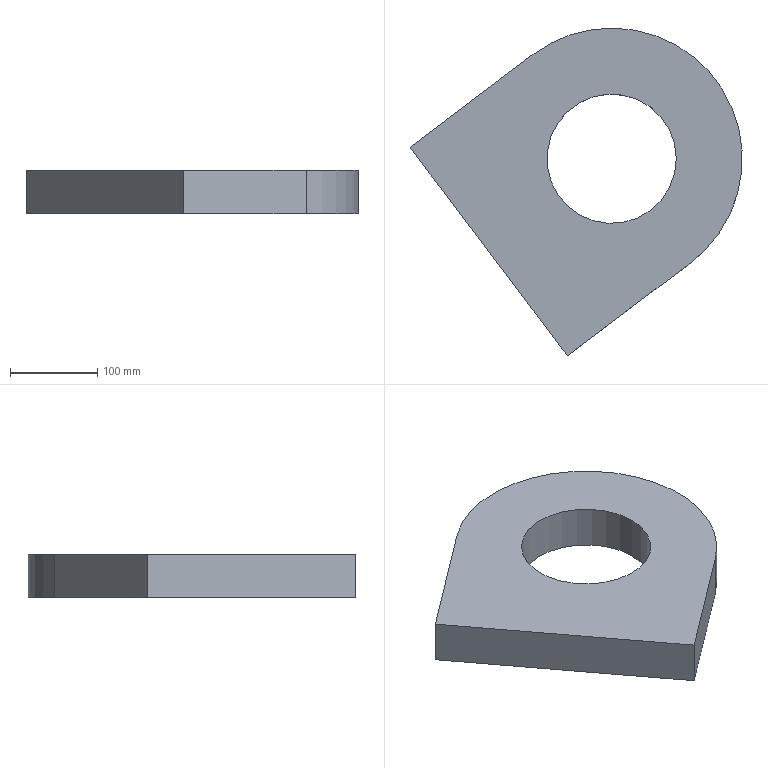Part | NX | features 底座(默认<按焊接>) 2 | 1 solid | 7 faces | box 381.454 x 376.184 x 50 mm | volume 3554006 mm3 | plane 5 | cylinder 2 | commonest cylinder face diameters 148.4 x1 300 x1
STEP:
#1=CARTESIAN_POINT('',(2456.913,471.615,-412.));
#2=VERTEX_POINT('',#1);
#3=CARTESIAN_POINT('',(2637.457,232.025,-412.));
#4=VERTEX_POINT('',#3);
#5=CARTESIAN_POINT('',(2547.185,351.82,-412.));
#6=DIRECTION('',(0.,0.,-1.));
#7=DIRECTION('',(-1.,0.,0.));
#8=AXIS2_PLACEMENT_3D('',#5,#6,#7);
#9=CIRCLE('',#8,150.);
#10=EDGE_CURVE('',#2,#4,#9,.T.);
#11=ORIENTED_EDGE('',*,*,#10,.T.);
#12=CARTESIAN_POINT('',(2637.457,232.025,-462.));
#13=VERTEX_POINT('',#12);
#14=CARTESIAN_POINT('',(2637.457,232.025,-462.));
#15=DIRECTION('',(0.,0.,1.));
#16=VECTOR('',#15,1000.);
#17=LINE('',#14,#16);
#18=EDGE_CURVE('',#13,#4,#17,.T.);
#19=ORIENTED_EDGE('',*,*,#18,.F.);
#20=CARTESIAN_POINT('',(2456.913,471.615,-462.));
#21=VERTEX_POINT('',#20);
#22=CARTESIAN_POINT('',(2547.185,351.82,-462.));
#23=DIRECTION('',(0.,0.,-1.));
#24=DIRECTION('',(-1.,0.,0.));
#25=AXIS2_PLACEMENT_3D('',#22,#23,#24);
#26=CIRCLE('',#25,150.);
#27=EDGE_CURVE('',#21,#13,#26,.T.);
#28=ORIENTED_EDGE('',*,*,#27,.F.);
#29=CARTESIAN_POINT('',(2456.913,471.615,-462.));
#30=DIRECTION('',(0.,0.,1.));
#31=VECTOR('',#30,1000.);
#32=LINE('',#29,#31);
#33=EDGE_CURVE('',#21,#2,#32,.T.);
#34=ORIENTED_EDGE('',*,*,#33,.T.);
#35=EDGE_LOOP('',(#11,#19,#28,#34));
#36=FACE_BOUND('',#35,.T.);
#37=CARTESIAN_POINT('',(2547.185,351.82,-462.));
#38=DIRECTION('',(0.,0.,1.));
#39=DIRECTION('',(1.,0.,0.));
#40=AXIS2_PLACEMENT_3D('',#37,#38,#39);
#41=CYLINDRICAL_SURFACE('',#40,150.);
#42=ADVANCED_FACE('',(#36),#41,.T.);
#43=CARTESIAN_POINT('',(2496.276,125.636,-412.));
#44=VERTEX_POINT('',#43);
#45=CARTESIAN_POINT('',(2637.457,232.025,-412.));
#46=DIRECTION('',(-0.7986,-0.6018,0.));
#47=VECTOR('',#46,1000.);
#48=LINE('',#45,#47);
#49=EDGE_CURVE('',#4,#44,#48,.T.);
#50=ORIENTED_EDGE('',*,*,#49,.T.);
#51=CARTESIAN_POINT('',(2496.276,125.636,-462.));
#52=VERTEX_POINT('',#51);
#53=CARTESIAN_POINT('',(2496.276,125.636,-462.));
#54=DIRECTION('',(0.,0.,1.));
#55=VECTOR('',#54,1000.);
#56=LINE('',#53,#55);
#57=EDGE_CURVE('',#52,#44,#56,.T.);
#58=ORIENTED_EDGE('',*,*,#57,.F.);
#59=CARTESIAN_POINT('',(2637.457,232.025,-462.));
#60=DIRECTION('',(-0.7986,-0.6018,0.));
#61=VECTOR('',#60,1000.);
#62=LINE('',#59,#61);
#63=EDGE_CURVE('',#13,#52,#62,.T.);
#64=ORIENTED_EDGE('',*,*,#63,.F.);
#65=ORIENTED_EDGE('',*,*,#18,.T.);
#66=EDGE_LOOP('',(#50,#58,#64,#65));
#67=FACE_BOUND('',#66,.T.);
#68=CARTESIAN_POINT('',(2637.457,232.025,-462.));
#69=DIRECTION('',(-0.6018,0.7986,0.));
#70=DIRECTION('',(-0.7986,-0.6018,0.));
#71=AXIS2_PLACEMENT_3D('',#68,#69,#70);
#72=PLANE('',#71);
#73=ADVANCED_FACE('',(#67),#72,.F.);
#74=CARTESIAN_POINT('',(2315.731,365.227,-412.));
#75=VERTEX_POINT('',#74);
#76=CARTESIAN_POINT('',(2315.731,365.227,-412.));
#77=DIRECTION('',(-0.6018,0.7986,0.));
#78=VECTOR('',#77,1000.);
#79=LINE('',#76,#78);
#80=EDGE_CURVE('',#44,#75,#79,.T.);
#81=ORIENTED_EDGE('',*,*,#80,.T.);
#82=CARTESIAN_POINT('',(2315.731,365.227,-462.));
#83=VERTEX_POINT('',#82);
#84=CARTESIAN_POINT('',(2315.731,365.227,-462.));
#85=DIRECTION('',(0.,0.,1.));
#86=VECTOR('',#85,1000.);
#87=LINE('',#84,#86);
#88=EDGE_CURVE('',#83,#75,#87,.T.);
#89=ORIENTED_EDGE('',*,*,#88,.F.);
#90=CARTESIAN_POINT('',(2315.731,365.227,-462.));
#91=DIRECTION('',(-0.6018,0.7986,0.));
#92=VECTOR('',#91,1000.);
#93=LINE('',#90,#92);
#94=EDGE_CURVE('',#52,#83,#93,.T.);
#95=ORIENTED_EDGE('',*,*,#94,.F.);
#96=ORIENTED_EDGE('',*,*,#57,.T.);
#97=EDGE_LOOP('',(#81,#89,#95,#96));
#98=FACE_BOUND('',#97,.T.);
#99=CARTESIAN_POINT('',(2315.731,365.227,-462.));
#100=DIRECTION('',(0.7986,0.6018,0.));
#101=DIRECTION('',(-0.6018,0.7986,0.));
#102=AXIS2_PLACEMENT_3D('',#99,#100,#101);
#103=PLANE('',#102);
#104=ADVANCED_FACE('',(#98),#103,.F.);
#105=CARTESIAN_POINT('',(2456.913,471.615,-412.));
#106=DIRECTION('',(0.7986,0.6018,0.));
#107=VECTOR('',#106,1000.);
#108=LINE('',#105,#107);
#109=EDGE_CURVE('',#75,#2,#108,.T.);
#110=ORIENTED_EDGE('',*,*,#109,.T.);
#111=ORIENTED_EDGE('',*,*,#33,.F.);
#112=CARTESIAN_POINT('',(2456.913,471.615,-462.));
#113=DIRECTION('',(0.7986,0.6018,0.));
#114=VECTOR('',#113,1000.);
#115=LINE('',#112,#114);
#116=EDGE_CURVE('',#83,#21,#115,.T.);
#117=ORIENTED_EDGE('',*,*,#116,.F.);
#118=ORIENTED_EDGE('',*,*,#88,.T.);
#119=EDGE_LOOP('',(#110,#111,#117,#118));
#120=FACE_BOUND('',#119,.T.);
#121=CARTESIAN_POINT('',(2456.913,471.615,-462.));
#122=DIRECTION('',(0.6018,-0.7986,0.));
#123=DIRECTION('',(0.7986,0.6018,0.));
#124=AXIS2_PLACEMENT_3D('',#121,#122,#123);
#125=PLANE('',#124);
#126=ADVANCED_FACE('',(#120),#125,.F.);
#127=CARTESIAN_POINT('',(2621.385,351.82,-462.));
#128=VERTEX_POINT('',#127);
#129=CARTESIAN_POINT('',(2547.185,351.82,-462.));
#130=DIRECTION('',(0.,0.,1.));
#131=DIRECTION('',(1.,0.,0.));
#132=AXIS2_PLACEMENT_3D('',#129,#130,#131);
#133=CIRCLE('',#132,74.2);
#134=EDGE_CURVE('',#128,#128,#133,.T.);
#135=ORIENTED_EDGE('',*,*,#134,.T.);
#136=EDGE_LOOP('',(#135));
#137=FACE_BOUND('',#136,.T.);
#138=ORIENTED_EDGE('',*,*,#27,.T.);
#139=ORIENTED_EDGE('',*,*,#63,.T.);
#140=ORIENTED_EDGE('',*,*,#94,.T.);
#141=ORIENTED_EDGE('',*,*,#116,.T.);
#142=EDGE_LOOP('',(#138,#139,#140,#141));
#143=FACE_BOUND('',#142,.T.);
#144=CARTESIAN_POINT('',(2547.185,351.82,-462.));
#145=DIRECTION('',(0.,0.,-1.));
#146=DIRECTION('',(-1.,0.,0.));
#147=AXIS2_PLACEMENT_3D('',#144,#145,#146);
#148=PLANE('',#147);
#149=ADVANCED_FACE('',(#137,#143),#148,.T.);
#150=CARTESIAN_POINT('',(2621.385,351.82,-412.));
#151=VERTEX_POINT('',#150);
#152=CARTESIAN_POINT('',(2547.185,351.82,-412.));
#153=DIRECTION('',(0.,0.,1.));
#154=DIRECTION('',(1.,0.,0.));
#155=AXIS2_PLACEMENT_3D('',#152,#153,#154);
#156=CIRCLE('',#155,74.2);
#157=EDGE_CURVE('',#151,#151,#156,.T.);
#158=ORIENTED_EDGE('',*,*,#157,.F.);
#159=EDGE_LOOP('',(#158));
#160=FACE_BOUND('',#159,.T.);
#161=ORIENTED_EDGE('',*,*,#10,.F.);
#162=ORIENTED_EDGE('',*,*,#109,.F.);
#163=ORIENTED_EDGE('',*,*,#80,.F.);
#164=ORIENTED_EDGE('',*,*,#49,.F.);
#165=EDGE_LOOP('',(#161,#162,#163,#164));
#166=FACE_BOUND('',#165,.T.);
#167=CARTESIAN_POINT('',(2547.185,351.82,-412.));
#168=DIRECTION('',(0.,0.,-1.));
#169=DIRECTION('',(-1.,0.,0.));
#170=AXIS2_PLACEMENT_3D('',#167,#168,#169);
#171=PLANE('',#170);
#172=ADVANCED_FACE('',(#160,#166),#171,.F.);
#173=ORIENTED_EDGE('',*,*,#134,.F.);
#174=EDGE_LOOP('',(#173));
#175=FACE_BOUND('',#174,.T.);
#176=ORIENTED_EDGE('',*,*,#157,.T.);
#177=EDGE_LOOP('',(#176));
#178=FACE_BOUND('',#177,.T.);
#179=CARTESIAN_POINT('',(2547.185,351.82,-396.));
#180=DIRECTION('',(0.,0.,-1.));
#181=DIRECTION('',(1.,0.,0.));
#182=AXIS2_PLACEMENT_3D('',#179,#180,#181);
#183=CYLINDRICAL_SURFACE('',#182,74.2);
#184=ADVANCED_FACE('',(#175,#178),#183,.F.);
#185=CLOSED_SHELL('',(#42,#73,#104,#126,#149,#172,#184));
#186=MANIFOLD_SOLID_BREP('',#185);
#187=(LENGTH_UNIT()NAMED_UNIT(*)SI_UNIT(.MILLI.,.METRE.));
#188=UNCERTAINTY_MEASURE_WITH_UNIT(LENGTH_MEASURE(0.00001),#187,'','');
#189=(NAMED_UNIT(*)PLANE_ANGLE_UNIT()SI_UNIT($,.RADIAN.));
#190=(NAMED_UNIT(*)SI_UNIT($,.STERADIAN.)SOLID_ANGLE_UNIT());
#191=(GEOMETRIC_REPRESENTATION_CONTEXT(3)GLOBAL_UNCERTAINTY_ASSIGNED_CONTEXT((#188))GLOBAL_UNIT_ASSIGNED_CONTEXT((#187,#189,#190))REPRESENTATION_CONTEXT('',''));
#192=ADVANCED_BREP_SHAPE_REPRESENTATION('',(#186),#191);